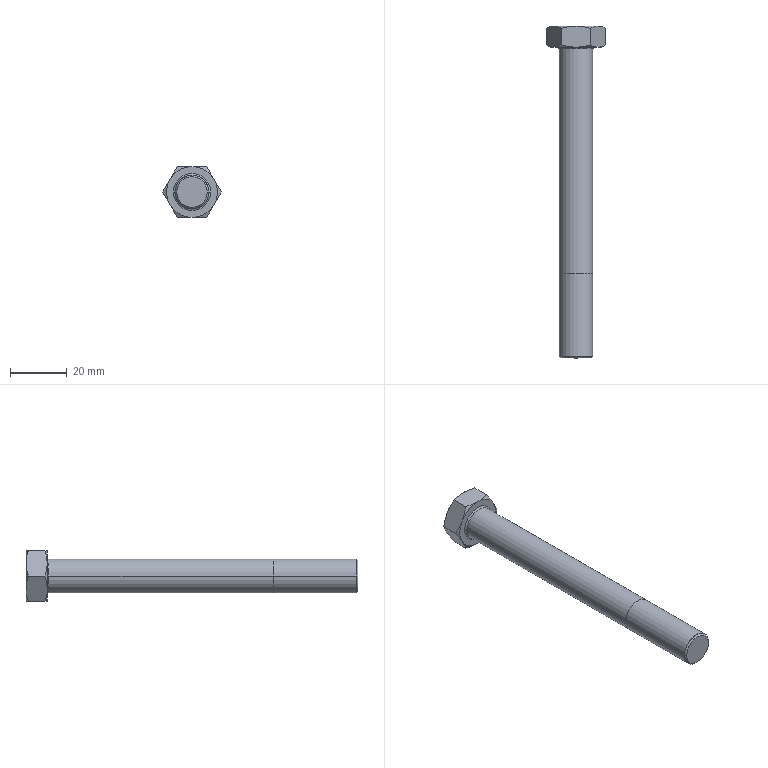Part | NX | features BREP 2 | 1 solid | 31 faces | box 20.785 x 117.5 x 18 mm | volume 15779 mm3 | cone 14 | plane 11 | cylinder 4 | torus 2 | commonest cylinder face diameters 10.106 x2 12 x2